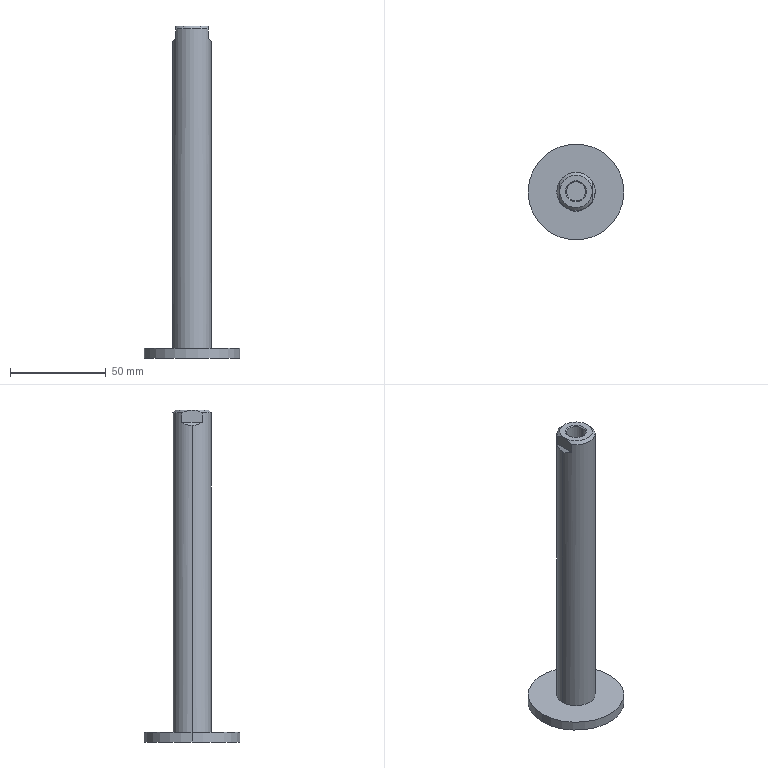Part | STEP file | CQ2A50-125DC-R06US_CQ22031Rods | 1 solid | 18 faces | box 50 x 50 x 173.25 mm | volume 61293 mm3 | plane 8 | cylinder 6 | cone 4 | commonest cylinder face diameters 10 x2 20 x2 50 x2